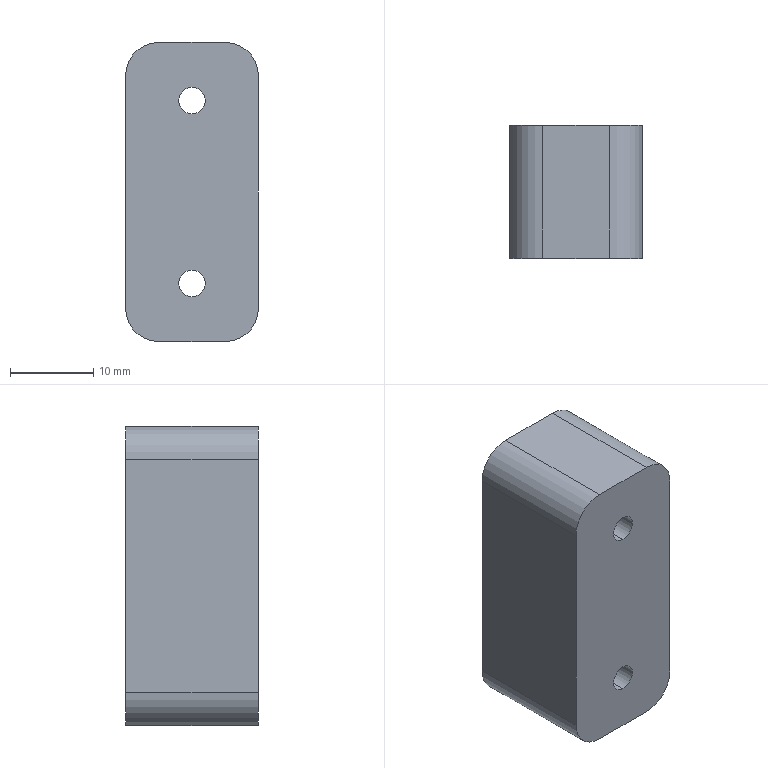Part | SolidWorks | features BaseBody 1 | 1 solid | 14 faces | box 16 x 16 x 36 mm | volume 8739 mm3 | cylinder 8 | plane 6 | commonest cylinder face diameters 3.2 x4 8 x4
STEP:
#1=CARTESIAN_POINT('',(0.,0.,12.6));
#2=VERTEX_POINT('',#1);
#3=CARTESIAN_POINT('',(0.,0.,9.4));
#4=VERTEX_POINT('',#3);
#5=CARTESIAN_POINT('',(0.,0.,11.));
#6=DIRECTION('',(0.,-1.,0.));
#7=DIRECTION('',(0.,0.,1.));
#8=AXIS2_PLACEMENT_3D('',#5,#6,#7);
#9=CIRCLE('',#8,1.6);
#10=EDGE_CURVE('',#2,#4,#9,.T.);
#11=ORIENTED_EDGE('',*,*,#10,.T.);
#12=CARTESIAN_POINT('',(0.,16.,9.4));
#13=VERTEX_POINT('',#12);
#14=CARTESIAN_POINT('',(0.,0.,9.4));
#15=DIRECTION('',(0.,1.,0.));
#16=VECTOR('',#15,1000.);
#17=LINE('',#14,#16);
#18=EDGE_CURVE('',#4,#13,#17,.T.);
#19=ORIENTED_EDGE('',*,*,#18,.T.);
#20=CARTESIAN_POINT('',(0.,16.,12.6));
#21=VERTEX_POINT('',#20);
#22=CARTESIAN_POINT('',(0.,16.,11.));
#23=DIRECTION('',(0.,-1.,0.));
#24=DIRECTION('',(0.,0.,1.));
#25=AXIS2_PLACEMENT_3D('',#22,#23,#24);
#26=CIRCLE('',#25,1.6);
#27=EDGE_CURVE('',#21,#13,#26,.T.);
#28=ORIENTED_EDGE('',*,*,#27,.F.);
#29=CARTESIAN_POINT('',(0.,0.,12.6));
#30=DIRECTION('',(0.,1.,0.));
#31=VECTOR('',#30,1000.);
#32=LINE('',#29,#31);
#33=EDGE_CURVE('',#2,#21,#32,.T.);
#34=ORIENTED_EDGE('',*,*,#33,.F.);
#35=EDGE_LOOP('',(#11,#19,#28,#34));
#36=FACE_OUTER_BOUND('',#35,.T.);
#37=CARTESIAN_POINT('',(0.,0.,11.));
#38=DIRECTION('',(0.,1.,0.));
#39=DIRECTION('',(0.,0.,1.));
#40=AXIS2_PLACEMENT_3D('',#37,#38,#39);
#41=CYLINDRICAL_SURFACE('',#40,1.6);
#42=ADVANCED_FACE('',(#36),#41,.F.);
#43=CARTESIAN_POINT('',(0.,0.,-9.4));
#44=VERTEX_POINT('',#43);
#45=CARTESIAN_POINT('',(0.,0.,-12.6));
#46=VERTEX_POINT('',#45);
#47=CARTESIAN_POINT('',(0.,0.,-11.));
#48=DIRECTION('',(0.,-1.,0.));
#49=DIRECTION('',(0.,0.,1.));
#50=AXIS2_PLACEMENT_3D('',#47,#48,#49);
#51=CIRCLE('',#50,1.6);
#52=EDGE_CURVE('',#44,#46,#51,.T.);
#53=ORIENTED_EDGE('',*,*,#52,.T.);
#54=CARTESIAN_POINT('',(0.,16.,-12.6));
#55=VERTEX_POINT('',#54);
#56=CARTESIAN_POINT('',(0.,0.,-12.6));
#57=DIRECTION('',(0.,1.,0.));
#58=VECTOR('',#57,1000.);
#59=LINE('',#56,#58);
#60=EDGE_CURVE('',#46,#55,#59,.T.);
#61=ORIENTED_EDGE('',*,*,#60,.T.);
#62=CARTESIAN_POINT('',(0.,16.,-9.4));
#63=VERTEX_POINT('',#62);
#64=CARTESIAN_POINT('',(0.,16.,-11.));
#65=DIRECTION('',(0.,-1.,0.));
#66=DIRECTION('',(0.,0.,1.));
#67=AXIS2_PLACEMENT_3D('',#64,#65,#66);
#68=CIRCLE('',#67,1.6);
#69=EDGE_CURVE('',#63,#55,#68,.T.);
#70=ORIENTED_EDGE('',*,*,#69,.F.);
#71=CARTESIAN_POINT('',(0.,0.,-9.4));
#72=DIRECTION('',(0.,1.,0.));
#73=VECTOR('',#72,1000.);
#74=LINE('',#71,#73);
#75=EDGE_CURVE('',#44,#63,#74,.T.);
#76=ORIENTED_EDGE('',*,*,#75,.F.);
#77=EDGE_LOOP('',(#53,#61,#70,#76));
#78=FACE_OUTER_BOUND('',#77,.T.);
#79=CARTESIAN_POINT('',(0.,0.,-11.));
#80=DIRECTION('',(0.,1.,0.));
#81=DIRECTION('',(0.,0.,1.));
#82=AXIS2_PLACEMENT_3D('',#79,#80,#81);
#83=CYLINDRICAL_SURFACE('',#82,1.6);
#84=ADVANCED_FACE('',(#78),#83,.F.);
#85=CARTESIAN_POINT('',(-4.,0.,-18.));
#86=VERTEX_POINT('',#85);
#87=CARTESIAN_POINT('',(-8.,0.,-14.));
#88=VERTEX_POINT('',#87);
#89=CARTESIAN_POINT('',(-4.,0.,-14.));
#90=DIRECTION('',(0.,1.,0.));
#91=DIRECTION('',(0.,0.,-1.));
#92=AXIS2_PLACEMENT_3D('',#89,#90,#91);
#93=CIRCLE('',#92,4.);
#94=EDGE_CURVE('',#86,#88,#93,.T.);
#95=ORIENTED_EDGE('',*,*,#94,.F.);
#96=CARTESIAN_POINT('',(4.,0.,-18.));
#97=VERTEX_POINT('',#96);
#98=CARTESIAN_POINT('',(0.,0.,-18.));
#99=DIRECTION('',(-1.,0.,0.));
#100=VECTOR('',#99,1000.);
#101=LINE('',#98,#100);
#102=EDGE_CURVE('',#97,#86,#101,.T.);
#103=ORIENTED_EDGE('',*,*,#102,.F.);
#104=CARTESIAN_POINT('',(8.,0.,-14.));
#105=VERTEX_POINT('',#104);
#106=CARTESIAN_POINT('',(4.,0.,-14.));
#107=DIRECTION('',(0.,1.,0.));
#108=DIRECTION('',(0.,0.,-1.));
#109=AXIS2_PLACEMENT_3D('',#106,#107,#108);
#110=CIRCLE('',#109,4.);
#111=EDGE_CURVE('',#105,#97,#110,.T.);
#112=ORIENTED_EDGE('',*,*,#111,.F.);
#113=CARTESIAN_POINT('',(8.,0.,14.));
#114=VERTEX_POINT('',#113);
#115=CARTESIAN_POINT('',(8.,0.,0.));
#116=DIRECTION('',(0.,0.,-1.));
#117=VECTOR('',#116,1000.);
#118=LINE('',#115,#117);
#119=EDGE_CURVE('',#114,#105,#118,.T.);
#120=ORIENTED_EDGE('',*,*,#119,.F.);
#121=CARTESIAN_POINT('',(4.,0.,18.));
#122=VERTEX_POINT('',#121);
#123=CARTESIAN_POINT('',(4.,0.,14.));
#124=DIRECTION('',(0.,1.,0.));
#125=DIRECTION('',(0.,0.,-1.));
#126=AXIS2_PLACEMENT_3D('',#123,#124,#125);
#127=CIRCLE('',#126,4.);
#128=EDGE_CURVE('',#122,#114,#127,.T.);
#129=ORIENTED_EDGE('',*,*,#128,.F.);
#130=CARTESIAN_POINT('',(-4.,0.,18.));
#131=VERTEX_POINT('',#130);
#132=CARTESIAN_POINT('',(0.,0.,18.));
#133=DIRECTION('',(1.,0.,0.));
#134=VECTOR('',#133,1000.);
#135=LINE('',#132,#134);
#136=EDGE_CURVE('',#131,#122,#135,.T.);
#137=ORIENTED_EDGE('',*,*,#136,.F.);
#138=CARTESIAN_POINT('',(-8.,0.,14.));
#139=VERTEX_POINT('',#138);
#140=CARTESIAN_POINT('',(-4.,0.,14.));
#141=DIRECTION('',(0.,1.,0.));
#142=DIRECTION('',(0.,0.,-1.));
#143=AXIS2_PLACEMENT_3D('',#140,#141,#142);
#144=CIRCLE('',#143,4.);
#145=EDGE_CURVE('',#139,#131,#144,.T.);
#146=ORIENTED_EDGE('',*,*,#145,.F.);
#147=CARTESIAN_POINT('',(-8.,0.,0.));
#148=DIRECTION('',(0.,0.,1.));
#149=VECTOR('',#148,1000.);
#150=LINE('',#147,#149);
#151=EDGE_CURVE('',#88,#139,#150,.T.);
#152=ORIENTED_EDGE('',*,*,#151,.F.);
#153=EDGE_LOOP('',(#95,#103,#112,#120,#129,#137,#146,#152));
#154=FACE_OUTER_BOUND('',#153,.T.);
#155=ORIENTED_EDGE('',*,*,#10,.F.);
#156=CARTESIAN_POINT('',(0.,0.,11.));
#157=DIRECTION('',(0.,-1.,0.));
#158=DIRECTION('',(0.,0.,1.));
#159=AXIS2_PLACEMENT_3D('',#156,#157,#158);
#160=CIRCLE('',#159,1.6);
#161=EDGE_CURVE('',#4,#2,#160,.T.);
#162=ORIENTED_EDGE('',*,*,#161,.F.);
#163=EDGE_LOOP('',(#155,#162));
#164=FACE_BOUND('',#163,.T.);
#165=ORIENTED_EDGE('',*,*,#52,.F.);
#166=CARTESIAN_POINT('',(0.,0.,-11.));
#167=DIRECTION('',(0.,-1.,0.));
#168=DIRECTION('',(0.,0.,1.));
#169=AXIS2_PLACEMENT_3D('',#166,#167,#168);
#170=CIRCLE('',#169,1.6);
#171=EDGE_CURVE('',#46,#44,#170,.T.);
#172=ORIENTED_EDGE('',*,*,#171,.F.);
#173=EDGE_LOOP('',(#165,#172));
#174=FACE_BOUND('',#173,.T.);
#175=CARTESIAN_POINT('',(0.,0.,0.));
#176=DIRECTION('',(0.,1.,0.));
#177=DIRECTION('',(0.,0.,1.));
#178=AXIS2_PLACEMENT_3D('',#175,#176,#177);
#179=PLANE('',#178);
#180=ADVANCED_FACE('',(#154,#164,#174),#179,.F.);
#181=CARTESIAN_POINT('',(-8.,16.,-14.));
#182=VERTEX_POINT('',#181);
#183=CARTESIAN_POINT('',(-8.,16.,-14.));
#184=DIRECTION('',(0.,1.,0.));
#185=VECTOR('',#184,1000.);
#186=LINE('',#183,#185);
#187=EDGE_CURVE('',#88,#182,#186,.T.);
#188=ORIENTED_EDGE('',*,*,#187,.F.);
#189=ORIENTED_EDGE('',*,*,#151,.T.);
#190=CARTESIAN_POINT('',(-8.,16.,14.));
#191=VERTEX_POINT('',#190);
#192=CARTESIAN_POINT('',(-8.,16.,14.));
#193=DIRECTION('',(0.,-1.,0.));
#194=VECTOR('',#193,1000.);
#195=LINE('',#192,#194);
#196=EDGE_CURVE('',#191,#139,#195,.T.);
#197=ORIENTED_EDGE('',*,*,#196,.F.);
#198=CARTESIAN_POINT('',(-8.,16.,18.));
#199=DIRECTION('',(0.,0.,1.));
#200=VECTOR('',#199,1000.);
#201=LINE('',#198,#200);
#202=EDGE_CURVE('',#182,#191,#201,.T.);
#203=ORIENTED_EDGE('',*,*,#202,.F.);
#204=EDGE_LOOP('',(#188,#189,#197,#203));
#205=FACE_OUTER_BOUND('',#204,.T.);
#206=CARTESIAN_POINT('',(-8.,16.,18.));
#207=DIRECTION('',(1.,0.,0.));
#208=DIRECTION('',(0.,0.,-1.));
#209=AXIS2_PLACEMENT_3D('',#206,#207,#208);
#210=PLANE('',#209);
#211=ADVANCED_FACE('',(#205),#210,.F.);
#212=ORIENTED_EDGE('',*,*,#94,.T.);
#213=ORIENTED_EDGE('',*,*,#187,.T.);
#214=CARTESIAN_POINT('',(-4.,16.,-18.));
#215=VERTEX_POINT('',#214);
#216=CARTESIAN_POINT('',(-4.,16.,-14.));
#217=DIRECTION('',(0.,-1.,0.));
#218=DIRECTION('',(0.,0.,-1.));
#219=AXIS2_PLACEMENT_3D('',#216,#217,#218);
#220=CIRCLE('',#219,4.);
#221=EDGE_CURVE('',#182,#215,#220,.T.);
#222=ORIENTED_EDGE('',*,*,#221,.T.);
#223=CARTESIAN_POINT('',(-4.,16.,-18.));
#224=DIRECTION('',(0.,-1.,0.));
#225=VECTOR('',#224,1000.);
#226=LINE('',#223,#225);
#227=EDGE_CURVE('',#215,#86,#226,.T.);
#228=ORIENTED_EDGE('',*,*,#227,.T.);
#229=EDGE_LOOP('',(#212,#213,#222,#228));
#230=FACE_OUTER_BOUND('',#229,.T.);
#231=CARTESIAN_POINT('',(-4.,16.,-14.));
#232=DIRECTION('',(0.,-1.,0.));
#233=DIRECTION('',(0.,0.,-1.));
#234=AXIS2_PLACEMENT_3D('',#231,#232,#233);
#235=CYLINDRICAL_SURFACE('',#234,4.);
#236=ADVANCED_FACE('',(#230),#235,.T.);
#237=ORIENTED_EDGE('',*,*,#227,.F.);
#238=CARTESIAN_POINT('',(4.,16.,-18.));
#239=VERTEX_POINT('',#238);
#240=CARTESIAN_POINT('',(8.,16.,-18.));
#241=DIRECTION('',(-1.,0.,0.));
#242=VECTOR('',#241,1000.);
#243=LINE('',#240,#242);
#244=EDGE_CURVE('',#239,#215,#243,.T.);
#245=ORIENTED_EDGE('',*,*,#244,.F.);
#246=CARTESIAN_POINT('',(4.,16.,-18.));
#247=DIRECTION('',(0.,1.,0.));
#248=VECTOR('',#247,1000.);
#249=LINE('',#246,#248);
#250=EDGE_CURVE('',#97,#239,#249,.T.);
#251=ORIENTED_EDGE('',*,*,#250,.F.);
#252=ORIENTED_EDGE('',*,*,#102,.T.);
#253=EDGE_LOOP('',(#237,#245,#251,#252));
#254=FACE_OUTER_BOUND('',#253,.T.);
#255=CARTESIAN_POINT('',(8.,16.,-18.));
#256=DIRECTION('',(0.,0.,1.));
#257=DIRECTION('',(1.,0.,0.));
#258=AXIS2_PLACEMENT_3D('',#255,#256,#257);
#259=PLANE('',#258);
#260=ADVANCED_FACE('',(#254),#259,.F.);
#261=ORIENTED_EDGE('',*,*,#111,.T.);
#262=ORIENTED_EDGE('',*,*,#250,.T.);
#263=CARTESIAN_POINT('',(8.,16.,-14.));
#264=VERTEX_POINT('',#263);
#265=CARTESIAN_POINT('',(4.,16.,-14.));
#266=DIRECTION('',(0.,-1.,0.));
#267=DIRECTION('',(0.,0.,-1.));
#268=AXIS2_PLACEMENT_3D('',#265,#266,#267);
#269=CIRCLE('',#268,4.);
#270=EDGE_CURVE('',#239,#264,#269,.T.);
#271=ORIENTED_EDGE('',*,*,#270,.T.);
#272=CARTESIAN_POINT('',(8.,16.,-14.));
#273=DIRECTION('',(0.,-1.,0.));
#274=VECTOR('',#273,1000.);
#275=LINE('',#272,#274);
#276=EDGE_CURVE('',#264,#105,#275,.T.);
#277=ORIENTED_EDGE('',*,*,#276,.T.);
#278=EDGE_LOOP('',(#261,#262,#271,#277));
#279=FACE_OUTER_BOUND('',#278,.T.);
#280=CARTESIAN_POINT('',(4.,16.,-14.));
#281=DIRECTION('',(0.,-1.,0.));
#282=DIRECTION('',(0.,0.,-1.));
#283=AXIS2_PLACEMENT_3D('',#280,#281,#282);
#284=CYLINDRICAL_SURFACE('',#283,4.);
#285=ADVANCED_FACE('',(#279),#284,.T.);
#286=ORIENTED_EDGE('',*,*,#276,.F.);
#287=CARTESIAN_POINT('',(8.,16.,14.));
#288=VERTEX_POINT('',#287);
#289=CARTESIAN_POINT('',(8.,16.,18.));
#290=DIRECTION('',(0.,0.,-1.));
#291=VECTOR('',#290,1000.);
#292=LINE('',#289,#291);
#293=EDGE_CURVE('',#288,#264,#292,.T.);
#294=ORIENTED_EDGE('',*,*,#293,.F.);
#295=CARTESIAN_POINT('',(8.,16.,14.));
#296=DIRECTION('',(0.,1.,0.));
#297=VECTOR('',#296,1000.);
#298=LINE('',#295,#297);
#299=EDGE_CURVE('',#114,#288,#298,.T.);
#300=ORIENTED_EDGE('',*,*,#299,.F.);
#301=ORIENTED_EDGE('',*,*,#119,.T.);
#302=EDGE_LOOP('',(#286,#294,#300,#301));
#303=FACE_OUTER_BOUND('',#302,.T.);
#304=CARTESIAN_POINT('',(8.,16.,18.));
#305=DIRECTION('',(-1.,0.,0.));
#306=DIRECTION('',(0.,0.,1.));
#307=AXIS2_PLACEMENT_3D('',#304,#305,#306);
#308=PLANE('',#307);
#309=ADVANCED_FACE('',(#303),#308,.F.);
#310=ORIENTED_EDGE('',*,*,#128,.T.);
#311=ORIENTED_EDGE('',*,*,#299,.T.);
#312=CARTESIAN_POINT('',(4.,16.,18.));
#313=VERTEX_POINT('',#312);
#314=CARTESIAN_POINT('',(4.,16.,14.));
#315=DIRECTION('',(0.,-1.,0.));
#316=DIRECTION('',(0.,0.,-1.));
#317=AXIS2_PLACEMENT_3D('',#314,#315,#316);
#318=CIRCLE('',#317,4.);
#319=EDGE_CURVE('',#288,#313,#318,.T.);
#320=ORIENTED_EDGE('',*,*,#319,.T.);
#321=CARTESIAN_POINT('',(4.,16.,18.));
#322=DIRECTION('',(0.,-1.,0.));
#323=VECTOR('',#322,1000.);
#324=LINE('',#321,#323);
#325=EDGE_CURVE('',#313,#122,#324,.T.);
#326=ORIENTED_EDGE('',*,*,#325,.T.);
#327=EDGE_LOOP('',(#310,#311,#320,#326));
#328=FACE_OUTER_BOUND('',#327,.T.);
#329=CARTESIAN_POINT('',(4.,16.,14.));
#330=DIRECTION('',(0.,-1.,0.));
#331=DIRECTION('',(0.,0.,-1.));
#332=AXIS2_PLACEMENT_3D('',#329,#330,#331);
#333=CYLINDRICAL_SURFACE('',#332,4.);
#334=ADVANCED_FACE('',(#328),#333,.T.);
#335=ORIENTED_EDGE('',*,*,#325,.F.);
#336=CARTESIAN_POINT('',(-4.,16.,18.));
#337=VERTEX_POINT('',#336);
#338=CARTESIAN_POINT('',(8.,16.,18.));
#339=DIRECTION('',(1.,0.,0.));
#340=VECTOR('',#339,1000.);
#341=LINE('',#338,#340);
#342=EDGE_CURVE('',#337,#313,#341,.T.);
#343=ORIENTED_EDGE('',*,*,#342,.F.);
#344=CARTESIAN_POINT('',(-4.,16.,18.));
#345=DIRECTION('',(0.,1.,0.));
#346=VECTOR('',#345,1000.);
#347=LINE('',#344,#346);
#348=EDGE_CURVE('',#131,#337,#347,.T.);
#349=ORIENTED_EDGE('',*,*,#348,.F.);
#350=ORIENTED_EDGE('',*,*,#136,.T.);
#351=EDGE_LOOP('',(#335,#343,#349,#350));
#352=FACE_OUTER_BOUND('',#351,.T.);
#353=CARTESIAN_POINT('',(8.,16.,18.));
#354=DIRECTION('',(0.,0.,-1.));
#355=DIRECTION('',(-1.,0.,0.));
#356=AXIS2_PLACEMENT_3D('',#353,#354,#355);
#357=PLANE('',#356);
#358=ADVANCED_FACE('',(#352),#357,.F.);
#359=ORIENTED_EDGE('',*,*,#145,.T.);
#360=ORIENTED_EDGE('',*,*,#348,.T.);
#361=CARTESIAN_POINT('',(-4.,16.,14.));
#362=DIRECTION('',(0.,-1.,0.));
#363=DIRECTION('',(0.,0.,-1.));
#364=AXIS2_PLACEMENT_3D('',#361,#362,#363);
#365=CIRCLE('',#364,4.);
#366=EDGE_CURVE('',#337,#191,#365,.T.);
#367=ORIENTED_EDGE('',*,*,#366,.T.);
#368=ORIENTED_EDGE('',*,*,#196,.T.);
#369=EDGE_LOOP('',(#359,#360,#367,#368));
#370=FACE_OUTER_BOUND('',#369,.T.);
#371=CARTESIAN_POINT('',(-4.,16.,14.));
#372=DIRECTION('',(0.,-1.,0.));
#373=DIRECTION('',(0.,0.,-1.));
#374=AXIS2_PLACEMENT_3D('',#371,#372,#373);
#375=CYLINDRICAL_SURFACE('',#374,4.);
#376=ADVANCED_FACE('',(#370),#375,.T.);
#377=ORIENTED_EDGE('',*,*,#18,.F.);
#378=ORIENTED_EDGE('',*,*,#161,.T.);
#379=ORIENTED_EDGE('',*,*,#33,.T.);
#380=CARTESIAN_POINT('',(0.,16.,11.));
#381=DIRECTION('',(0.,-1.,0.));
#382=DIRECTION('',(0.,0.,1.));
#383=AXIS2_PLACEMENT_3D('',#380,#381,#382);
#384=CIRCLE('',#383,1.6);
#385=EDGE_CURVE('',#13,#21,#384,.T.);
#386=ORIENTED_EDGE('',*,*,#385,.F.);
#387=EDGE_LOOP('',(#377,#378,#379,#386));
#388=FACE_OUTER_BOUND('',#387,.T.);
#389=CARTESIAN_POINT('',(0.,0.,11.));
#390=DIRECTION('',(0.,1.,0.));
#391=DIRECTION('',(0.,0.,1.));
#392=AXIS2_PLACEMENT_3D('',#389,#390,#391);
#393=CYLINDRICAL_SURFACE('',#392,1.6);
#394=ADVANCED_FACE('',(#388),#393,.F.);
#395=ORIENTED_EDGE('',*,*,#60,.F.);
#396=ORIENTED_EDGE('',*,*,#171,.T.);
#397=ORIENTED_EDGE('',*,*,#75,.T.);
#398=CARTESIAN_POINT('',(0.,16.,-11.));
#399=DIRECTION('',(0.,-1.,0.));
#400=DIRECTION('',(0.,0.,1.));
#401=AXIS2_PLACEMENT_3D('',#398,#399,#400);
#402=CIRCLE('',#401,1.6);
#403=EDGE_CURVE('',#55,#63,#402,.T.);
#404=ORIENTED_EDGE('',*,*,#403,.F.);
#405=EDGE_LOOP('',(#395,#396,#397,#404));
#406=FACE_OUTER_BOUND('',#405,.T.);
#407=CARTESIAN_POINT('',(0.,0.,-11.));
#408=DIRECTION('',(0.,1.,0.));
#409=DIRECTION('',(0.,0.,1.));
#410=AXIS2_PLACEMENT_3D('',#407,#408,#409);
#411=CYLINDRICAL_SURFACE('',#410,1.6);
#412=ADVANCED_FACE('',(#406),#411,.F.);
#413=ORIENTED_EDGE('',*,*,#293,.T.);
#414=ORIENTED_EDGE('',*,*,#270,.F.);
#415=ORIENTED_EDGE('',*,*,#244,.T.);
#416=ORIENTED_EDGE('',*,*,#221,.F.);
#417=ORIENTED_EDGE('',*,*,#202,.T.);
#418=ORIENTED_EDGE('',*,*,#366,.F.);
#419=ORIENTED_EDGE('',*,*,#342,.T.);
#420=ORIENTED_EDGE('',*,*,#319,.F.);
#421=EDGE_LOOP('',(#413,#414,#415,#416,#417,#418,#419,#420));
#422=FACE_OUTER_BOUND('',#421,.T.);
#423=ORIENTED_EDGE('',*,*,#27,.T.);
#424=ORIENTED_EDGE('',*,*,#385,.T.);
#425=EDGE_LOOP('',(#423,#424));
#426=FACE_BOUND('',#425,.T.);
#427=ORIENTED_EDGE('',*,*,#69,.T.);
#428=ORIENTED_EDGE('',*,*,#403,.T.);
#429=EDGE_LOOP('',(#427,#428));
#430=FACE_BOUND('',#429,.T.);
#431=CARTESIAN_POINT('',(0.,16.,0.));
#432=DIRECTION('',(0.,1.,0.));
#433=DIRECTION('',(0.,0.,1.));
#434=AXIS2_PLACEMENT_3D('',#431,#432,#433);
#435=PLANE('',#434);
#436=ADVANCED_FACE('',(#422,#426,#430),#435,.T.);
#437=CLOSED_SHELL('',(#42,#84,#180,#211,#236,#260,#285,#309,#334,#358,#376,#394,#412,#436));
#438=MANIFOLD_SOLID_BREP('',#437);
#439=CARTESIAN_POINT('',(0.,0.,0.));
#440=DIRECTION('',(0.,0.,1.));
#441=DIRECTION('',(1.,0.,0.));
#442=AXIS2_PLACEMENT_3D('',#439,#440,#441);
#443=(LENGTH_UNIT()NAMED_UNIT(*)SI_UNIT(.MILLI.,.METRE.));
#444=UNCERTAINTY_MEASURE_WITH_UNIT(LENGTH_MEASURE(0.00001),#443,'','');
#445=(NAMED_UNIT(*)PLANE_ANGLE_UNIT()SI_UNIT($,.RADIAN.));
#446=(NAMED_UNIT(*)SI_UNIT($,.STERADIAN.)SOLID_ANGLE_UNIT());
#447=(GEOMETRIC_REPRESENTATION_CONTEXT(3)GLOBAL_UNCERTAINTY_ASSIGNED_CONTEXT((#444))GLOBAL_UNIT_ASSIGNED_CONTEXT((#443,#445,#446))REPRESENTATION_CONTEXT('',''));
#448=ADVANCED_BREP_SHAPE_REPRESENTATION('',(#438,#442),#447);